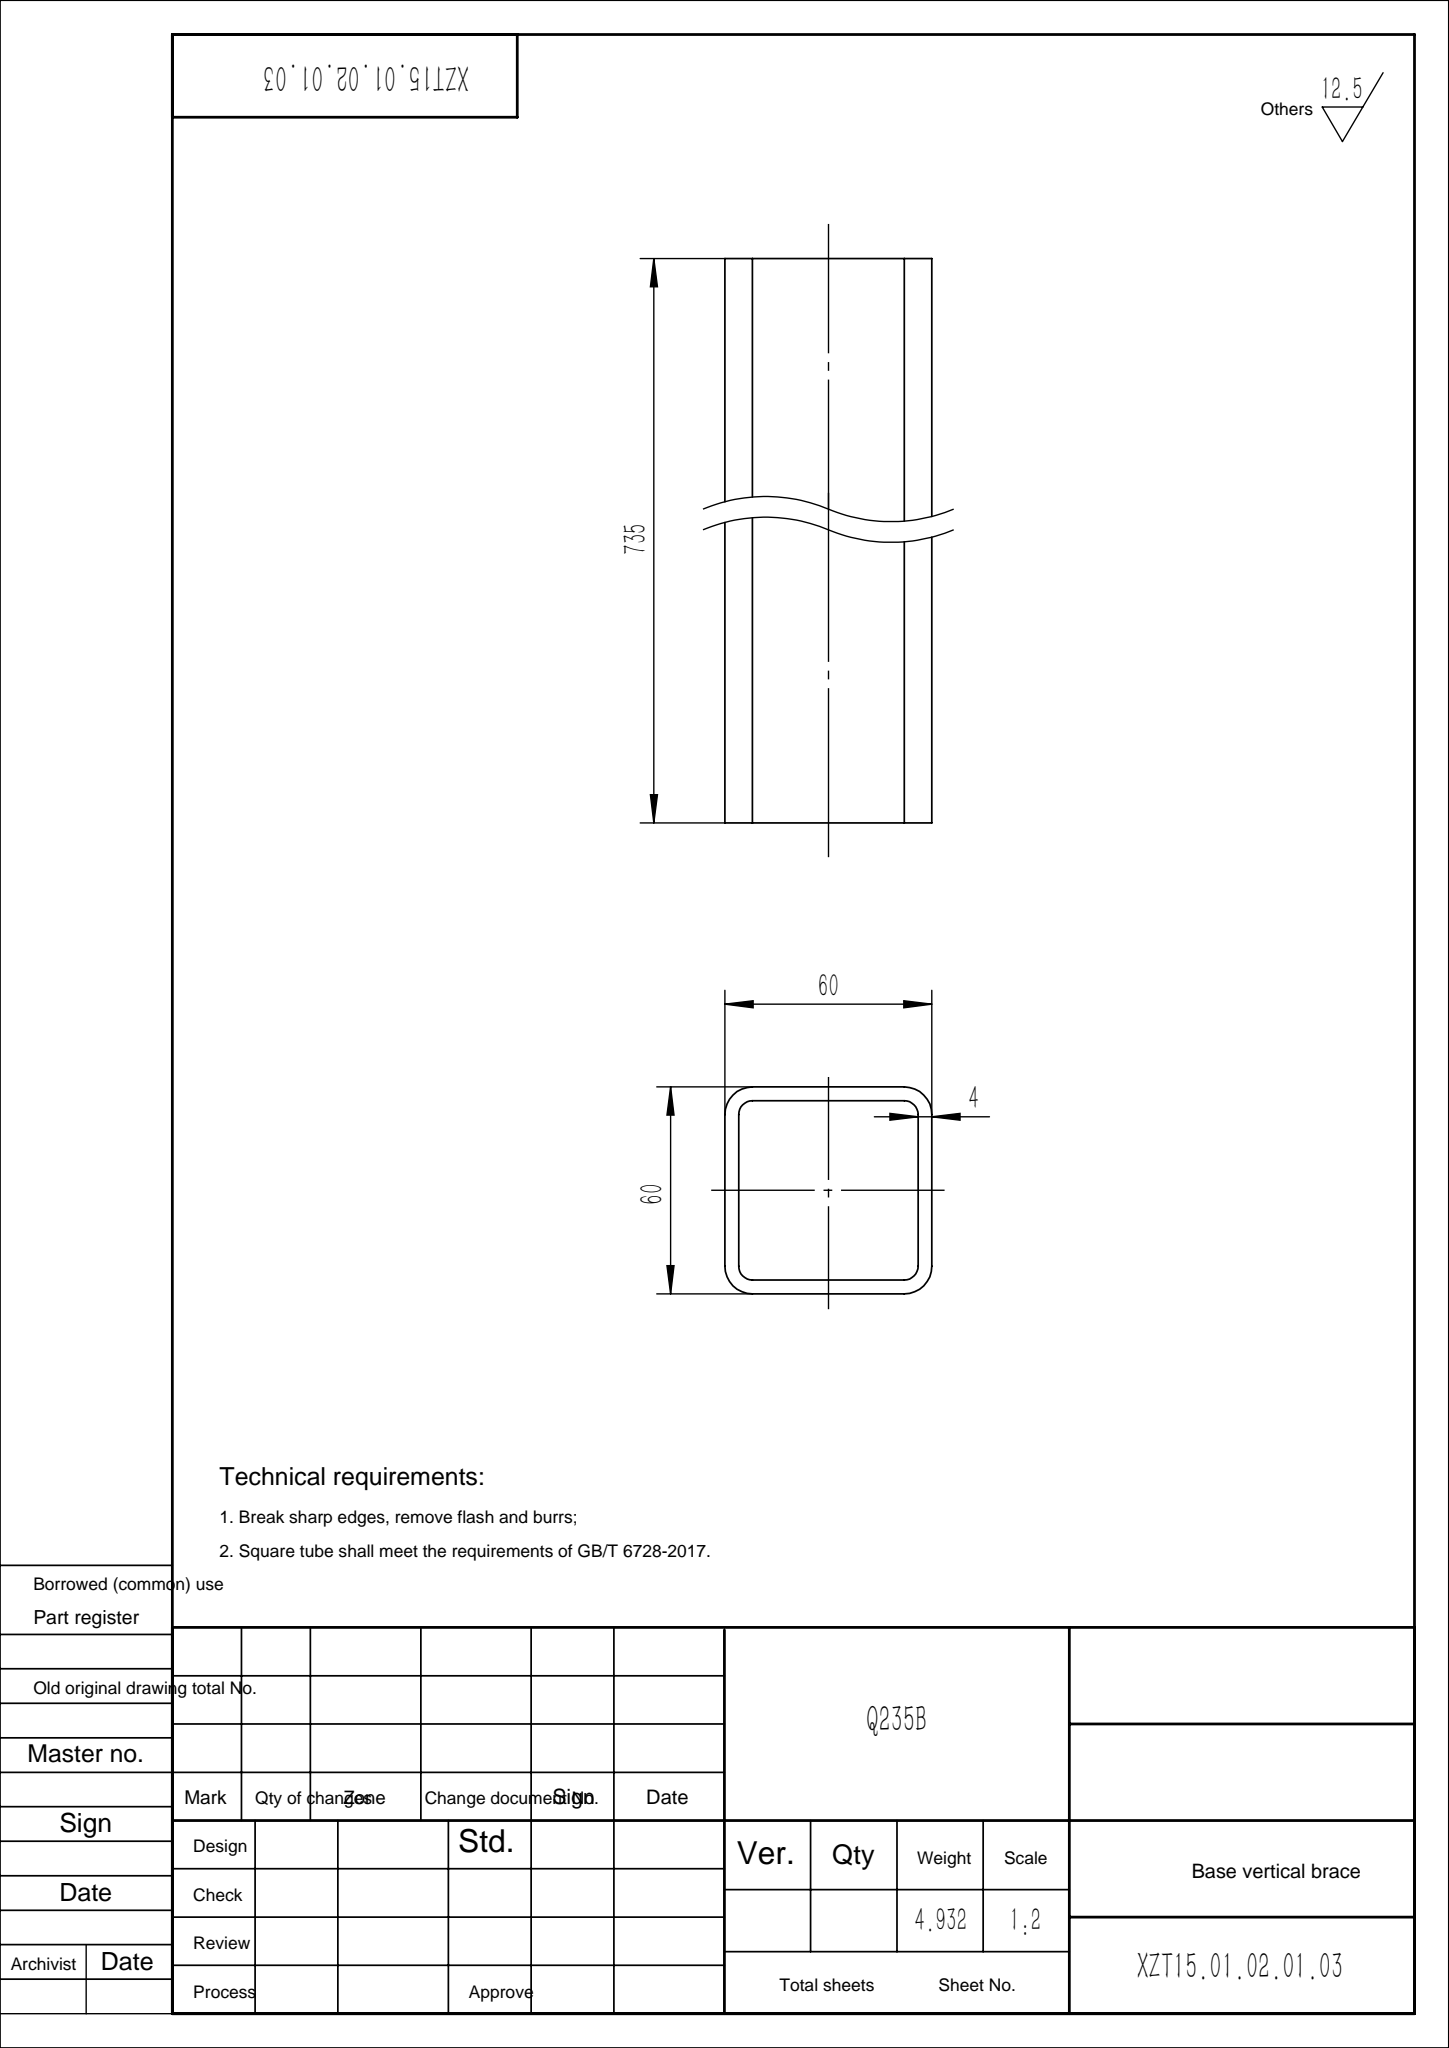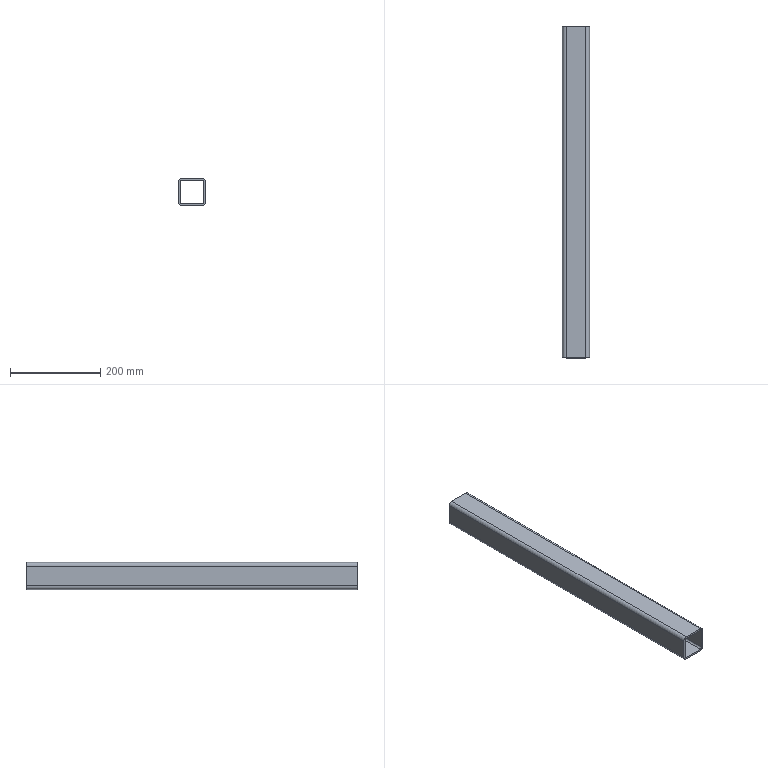Part | SolidWorks | features WeldMemberFeat 1, WeldmentFeature 1 | 1 solid | 18 faces | box 60 x 735 x 60 mm | volume 628275 mm3 | plane 10 | cylinder 8 | commonest cylinder face diameters 8 x4 16 x4
STEP:
#1=CARTESIAN_POINT('',(-30.,0.,22.));
#2=VERTEX_POINT('',#1);
#3=CARTESIAN_POINT('',(-22.,0.,30.));
#4=VERTEX_POINT('',#3);
#5=CARTESIAN_POINT('',(-22.,0.,22.));
#6=DIRECTION('',(0.,1.,0.));
#7=DIRECTION('',(0.,0.,1.));
#8=AXIS2_PLACEMENT_3D('',#5,#6,#7);
#9=CIRCLE('',#8,8.);
#10=EDGE_CURVE('',#2,#4,#9,.T.);
#11=ORIENTED_EDGE('',*,*,#10,.T.);
#12=CARTESIAN_POINT('',(-22.,735.,30.));
#13=VERTEX_POINT('',#12);
#14=CARTESIAN_POINT('',(-22.,735.,30.));
#15=DIRECTION('',(0.,-1.,0.));
#16=VECTOR('',#15,1000.);
#17=LINE('',#14,#16);
#18=EDGE_CURVE('',#13,#4,#17,.T.);
#19=ORIENTED_EDGE('',*,*,#18,.F.);
#20=CARTESIAN_POINT('',(-30.,735.,22.));
#21=VERTEX_POINT('',#20);
#22=CARTESIAN_POINT('',(-22.,735.,22.));
#23=DIRECTION('',(0.,1.,0.));
#24=DIRECTION('',(0.,0.,1.));
#25=AXIS2_PLACEMENT_3D('',#22,#23,#24);
#26=CIRCLE('',#25,8.);
#27=EDGE_CURVE('',#21,#13,#26,.T.);
#28=ORIENTED_EDGE('',*,*,#27,.F.);
#29=CARTESIAN_POINT('',(-30.,735.,22.));
#30=DIRECTION('',(0.,-1.,0.));
#31=VECTOR('',#30,1000.);
#32=LINE('',#29,#31);
#33=EDGE_CURVE('',#21,#2,#32,.T.);
#34=ORIENTED_EDGE('',*,*,#33,.T.);
#35=EDGE_LOOP('',(#11,#19,#28,#34));
#36=FACE_OUTER_BOUND('',#35,.T.);
#37=CARTESIAN_POINT('',(-22.,735.,22.));
#38=DIRECTION('',(0.,-1.,0.));
#39=DIRECTION('',(0.,0.,-1.));
#40=AXIS2_PLACEMENT_3D('',#37,#38,#39);
#41=CYLINDRICAL_SURFACE('',#40,8.);
#42=ADVANCED_FACE('',(#36),#41,.T.);
#43=CARTESIAN_POINT('',(22.,0.,30.));
#44=VERTEX_POINT('',#43);
#45=CARTESIAN_POINT('',(-22.,0.,30.));
#46=DIRECTION('',(1.,0.,0.));
#47=VECTOR('',#46,1000.);
#48=LINE('',#45,#47);
#49=EDGE_CURVE('',#4,#44,#48,.T.);
#50=ORIENTED_EDGE('',*,*,#49,.T.);
#51=CARTESIAN_POINT('',(22.,735.,30.));
#52=VERTEX_POINT('',#51);
#53=CARTESIAN_POINT('',(22.,735.,30.));
#54=DIRECTION('',(0.,-1.,0.));
#55=VECTOR('',#54,1000.);
#56=LINE('',#53,#55);
#57=EDGE_CURVE('',#52,#44,#56,.T.);
#58=ORIENTED_EDGE('',*,*,#57,.F.);
#59=CARTESIAN_POINT('',(-22.,735.,30.));
#60=DIRECTION('',(1.,0.,0.));
#61=VECTOR('',#60,1000.);
#62=LINE('',#59,#61);
#63=EDGE_CURVE('',#13,#52,#62,.T.);
#64=ORIENTED_EDGE('',*,*,#63,.F.);
#65=ORIENTED_EDGE('',*,*,#18,.T.);
#66=EDGE_LOOP('',(#50,#58,#64,#65));
#67=FACE_OUTER_BOUND('',#66,.T.);
#68=CARTESIAN_POINT('',(-22.,735.,30.));
#69=DIRECTION('',(0.,0.,-1.));
#70=DIRECTION('',(-1.,0.,0.));
#71=AXIS2_PLACEMENT_3D('',#68,#69,#70);
#72=PLANE('',#71);
#73=ADVANCED_FACE('',(#67),#72,.F.);
#74=CARTESIAN_POINT('',(30.,0.,22.));
#75=VERTEX_POINT('',#74);
#76=CARTESIAN_POINT('',(22.,0.,22.));
#77=DIRECTION('',(0.,1.,0.));
#78=DIRECTION('',(0.,0.,1.));
#79=AXIS2_PLACEMENT_3D('',#76,#77,#78);
#80=CIRCLE('',#79,8.);
#81=EDGE_CURVE('',#44,#75,#80,.T.);
#82=ORIENTED_EDGE('',*,*,#81,.T.);
#83=CARTESIAN_POINT('',(30.,735.,22.));
#84=VERTEX_POINT('',#83);
#85=CARTESIAN_POINT('',(30.,735.,22.));
#86=DIRECTION('',(0.,-1.,0.));
#87=VECTOR('',#86,1000.);
#88=LINE('',#85,#87);
#89=EDGE_CURVE('',#84,#75,#88,.T.);
#90=ORIENTED_EDGE('',*,*,#89,.F.);
#91=CARTESIAN_POINT('',(22.,735.,22.));
#92=DIRECTION('',(0.,1.,0.));
#93=DIRECTION('',(0.,0.,1.));
#94=AXIS2_PLACEMENT_3D('',#91,#92,#93);
#95=CIRCLE('',#94,8.);
#96=EDGE_CURVE('',#52,#84,#95,.T.);
#97=ORIENTED_EDGE('',*,*,#96,.F.);
#98=ORIENTED_EDGE('',*,*,#57,.T.);
#99=EDGE_LOOP('',(#82,#90,#97,#98));
#100=FACE_OUTER_BOUND('',#99,.T.);
#101=CARTESIAN_POINT('',(22.,735.,22.));
#102=DIRECTION('',(0.,-1.,0.));
#103=DIRECTION('',(0.,0.,-1.));
#104=AXIS2_PLACEMENT_3D('',#101,#102,#103);
#105=CYLINDRICAL_SURFACE('',#104,8.);
#106=ADVANCED_FACE('',(#100),#105,.T.);
#107=CARTESIAN_POINT('',(30.,0.,-22.));
#108=VERTEX_POINT('',#107);
#109=CARTESIAN_POINT('',(30.,0.,-22.));
#110=DIRECTION('',(0.,0.,-1.));
#111=VECTOR('',#110,1000.);
#112=LINE('',#109,#111);
#113=EDGE_CURVE('',#75,#108,#112,.T.);
#114=ORIENTED_EDGE('',*,*,#113,.T.);
#115=CARTESIAN_POINT('',(30.,735.,-22.));
#116=VERTEX_POINT('',#115);
#117=CARTESIAN_POINT('',(30.,735.,-22.));
#118=DIRECTION('',(0.,-1.,0.));
#119=VECTOR('',#118,1000.);
#120=LINE('',#117,#119);
#121=EDGE_CURVE('',#116,#108,#120,.T.);
#122=ORIENTED_EDGE('',*,*,#121,.F.);
#123=CARTESIAN_POINT('',(30.,735.,-22.));
#124=DIRECTION('',(0.,0.,-1.));
#125=VECTOR('',#124,1000.);
#126=LINE('',#123,#125);
#127=EDGE_CURVE('',#84,#116,#126,.T.);
#128=ORIENTED_EDGE('',*,*,#127,.F.);
#129=ORIENTED_EDGE('',*,*,#89,.T.);
#130=EDGE_LOOP('',(#114,#122,#128,#129));
#131=FACE_OUTER_BOUND('',#130,.T.);
#132=CARTESIAN_POINT('',(30.,735.,-22.));
#133=DIRECTION('',(-1.,0.,0.));
#134=DIRECTION('',(0.,0.,1.));
#135=AXIS2_PLACEMENT_3D('',#132,#133,#134);
#136=PLANE('',#135);
#137=ADVANCED_FACE('',(#131),#136,.F.);
#138=CARTESIAN_POINT('',(22.,0.,-30.));
#139=VERTEX_POINT('',#138);
#140=CARTESIAN_POINT('',(22.,0.,-22.));
#141=DIRECTION('',(0.,1.,0.));
#142=DIRECTION('',(0.,0.,1.));
#143=AXIS2_PLACEMENT_3D('',#140,#141,#142);
#144=CIRCLE('',#143,8.);
#145=EDGE_CURVE('',#108,#139,#144,.T.);
#146=ORIENTED_EDGE('',*,*,#145,.T.);
#147=CARTESIAN_POINT('',(22.,735.,-30.));
#148=VERTEX_POINT('',#147);
#149=CARTESIAN_POINT('',(22.,735.,-30.));
#150=DIRECTION('',(0.,-1.,0.));
#151=VECTOR('',#150,1000.);
#152=LINE('',#149,#151);
#153=EDGE_CURVE('',#148,#139,#152,.T.);
#154=ORIENTED_EDGE('',*,*,#153,.F.);
#155=CARTESIAN_POINT('',(22.,735.,-22.));
#156=DIRECTION('',(0.,1.,0.));
#157=DIRECTION('',(0.,0.,1.));
#158=AXIS2_PLACEMENT_3D('',#155,#156,#157);
#159=CIRCLE('',#158,8.);
#160=EDGE_CURVE('',#116,#148,#159,.T.);
#161=ORIENTED_EDGE('',*,*,#160,.F.);
#162=ORIENTED_EDGE('',*,*,#121,.T.);
#163=EDGE_LOOP('',(#146,#154,#161,#162));
#164=FACE_OUTER_BOUND('',#163,.T.);
#165=CARTESIAN_POINT('',(22.,735.,-22.));
#166=DIRECTION('',(0.,-1.,0.));
#167=DIRECTION('',(0.,0.,-1.));
#168=AXIS2_PLACEMENT_3D('',#165,#166,#167);
#169=CYLINDRICAL_SURFACE('',#168,8.);
#170=ADVANCED_FACE('',(#164),#169,.T.);
#171=CARTESIAN_POINT('',(-22.,0.,-30.));
#172=VERTEX_POINT('',#171);
#173=CARTESIAN_POINT('',(22.,0.,-30.));
#174=DIRECTION('',(-1.,0.,0.));
#175=VECTOR('',#174,1000.);
#176=LINE('',#173,#175);
#177=EDGE_CURVE('',#139,#172,#176,.T.);
#178=ORIENTED_EDGE('',*,*,#177,.T.);
#179=CARTESIAN_POINT('',(-22.,735.,-30.));
#180=VERTEX_POINT('',#179);
#181=CARTESIAN_POINT('',(-22.,735.,-30.));
#182=DIRECTION('',(0.,-1.,0.));
#183=VECTOR('',#182,1000.);
#184=LINE('',#181,#183);
#185=EDGE_CURVE('',#180,#172,#184,.T.);
#186=ORIENTED_EDGE('',*,*,#185,.F.);
#187=CARTESIAN_POINT('',(22.,735.,-30.));
#188=DIRECTION('',(-1.,0.,0.));
#189=VECTOR('',#188,1000.);
#190=LINE('',#187,#189);
#191=EDGE_CURVE('',#148,#180,#190,.T.);
#192=ORIENTED_EDGE('',*,*,#191,.F.);
#193=ORIENTED_EDGE('',*,*,#153,.T.);
#194=EDGE_LOOP('',(#178,#186,#192,#193));
#195=FACE_OUTER_BOUND('',#194,.T.);
#196=CARTESIAN_POINT('',(22.,735.,-30.));
#197=DIRECTION('',(0.,0.,1.));
#198=DIRECTION('',(1.,0.,0.));
#199=AXIS2_PLACEMENT_3D('',#196,#197,#198);
#200=PLANE('',#199);
#201=ADVANCED_FACE('',(#195),#200,.F.);
#202=CARTESIAN_POINT('',(-30.,0.,-22.));
#203=VERTEX_POINT('',#202);
#204=CARTESIAN_POINT('',(-22.,0.,-22.));
#205=DIRECTION('',(0.,1.,0.));
#206=DIRECTION('',(0.,0.,1.));
#207=AXIS2_PLACEMENT_3D('',#204,#205,#206);
#208=CIRCLE('',#207,8.);
#209=EDGE_CURVE('',#172,#203,#208,.T.);
#210=ORIENTED_EDGE('',*,*,#209,.T.);
#211=CARTESIAN_POINT('',(-30.,735.,-22.));
#212=VERTEX_POINT('',#211);
#213=CARTESIAN_POINT('',(-30.,735.,-22.));
#214=DIRECTION('',(0.,-1.,0.));
#215=VECTOR('',#214,1000.);
#216=LINE('',#213,#215);
#217=EDGE_CURVE('',#212,#203,#216,.T.);
#218=ORIENTED_EDGE('',*,*,#217,.F.);
#219=CARTESIAN_POINT('',(-22.,735.,-22.));
#220=DIRECTION('',(0.,1.,0.));
#221=DIRECTION('',(0.,0.,1.));
#222=AXIS2_PLACEMENT_3D('',#219,#220,#221);
#223=CIRCLE('',#222,8.);
#224=EDGE_CURVE('',#180,#212,#223,.T.);
#225=ORIENTED_EDGE('',*,*,#224,.F.);
#226=ORIENTED_EDGE('',*,*,#185,.T.);
#227=EDGE_LOOP('',(#210,#218,#225,#226));
#228=FACE_OUTER_BOUND('',#227,.T.);
#229=CARTESIAN_POINT('',(-22.,735.,-22.));
#230=DIRECTION('',(0.,-1.,0.));
#231=DIRECTION('',(0.,0.,-1.));
#232=AXIS2_PLACEMENT_3D('',#229,#230,#231);
#233=CYLINDRICAL_SURFACE('',#232,8.);
#234=ADVANCED_FACE('',(#228),#233,.T.);
#235=CARTESIAN_POINT('',(22.,0.,26.));
#236=VERTEX_POINT('',#235);
#237=CARTESIAN_POINT('',(26.,0.,22.));
#238=VERTEX_POINT('',#237);
#239=CARTESIAN_POINT('',(22.,0.,22.));
#240=DIRECTION('',(0.,1.,0.));
#241=DIRECTION('',(0.,0.,1.));
#242=AXIS2_PLACEMENT_3D('',#239,#240,#241);
#243=CIRCLE('',#242,4.);
#244=EDGE_CURVE('',#236,#238,#243,.T.);
#245=ORIENTED_EDGE('',*,*,#244,.F.);
#246=CARTESIAN_POINT('',(22.,735.,26.));
#247=VERTEX_POINT('',#246);
#248=CARTESIAN_POINT('',(22.,735.,26.));
#249=DIRECTION('',(0.,-1.,0.));
#250=VECTOR('',#249,1000.);
#251=LINE('',#248,#250);
#252=EDGE_CURVE('',#247,#236,#251,.T.);
#253=ORIENTED_EDGE('',*,*,#252,.F.);
#254=CARTESIAN_POINT('',(26.,735.,22.));
#255=VERTEX_POINT('',#254);
#256=CARTESIAN_POINT('',(22.,735.,22.));
#257=DIRECTION('',(0.,1.,0.));
#258=DIRECTION('',(0.,0.,1.));
#259=AXIS2_PLACEMENT_3D('',#256,#257,#258);
#260=CIRCLE('',#259,4.);
#261=EDGE_CURVE('',#247,#255,#260,.T.);
#262=ORIENTED_EDGE('',*,*,#261,.T.);
#263=CARTESIAN_POINT('',(26.,735.,22.));
#264=DIRECTION('',(0.,-1.,0.));
#265=VECTOR('',#264,1000.);
#266=LINE('',#263,#265);
#267=EDGE_CURVE('',#255,#238,#266,.T.);
#268=ORIENTED_EDGE('',*,*,#267,.T.);
#269=EDGE_LOOP('',(#245,#253,#262,#268));
#270=FACE_OUTER_BOUND('',#269,.T.);
#271=CARTESIAN_POINT('',(22.,735.,22.));
#272=DIRECTION('',(0.,-1.,0.));
#273=DIRECTION('',(0.,0.,-1.));
#274=AXIS2_PLACEMENT_3D('',#271,#272,#273);
#275=CYLINDRICAL_SURFACE('',#274,4.);
#276=ADVANCED_FACE('',(#270),#275,.F.);
#277=CARTESIAN_POINT('',(-22.,0.,26.));
#278=VERTEX_POINT('',#277);
#279=CARTESIAN_POINT('',(-22.,0.,26.));
#280=DIRECTION('',(1.,0.,0.));
#281=VECTOR('',#280,1000.);
#282=LINE('',#279,#281);
#283=EDGE_CURVE('',#278,#236,#282,.T.);
#284=ORIENTED_EDGE('',*,*,#283,.F.);
#285=CARTESIAN_POINT('',(-22.,735.,26.));
#286=VERTEX_POINT('',#285);
#287=CARTESIAN_POINT('',(-22.,735.,26.));
#288=DIRECTION('',(0.,-1.,0.));
#289=VECTOR('',#288,1000.);
#290=LINE('',#287,#289);
#291=EDGE_CURVE('',#286,#278,#290,.T.);
#292=ORIENTED_EDGE('',*,*,#291,.F.);
#293=CARTESIAN_POINT('',(-22.,735.,26.));
#294=DIRECTION('',(1.,0.,0.));
#295=VECTOR('',#294,1000.);
#296=LINE('',#293,#295);
#297=EDGE_CURVE('',#286,#247,#296,.T.);
#298=ORIENTED_EDGE('',*,*,#297,.T.);
#299=ORIENTED_EDGE('',*,*,#252,.T.);
#300=EDGE_LOOP('',(#284,#292,#298,#299));
#301=FACE_OUTER_BOUND('',#300,.T.);
#302=CARTESIAN_POINT('',(-22.,735.,26.));
#303=DIRECTION('',(0.,0.,-1.));
#304=DIRECTION('',(-1.,0.,0.));
#305=AXIS2_PLACEMENT_3D('',#302,#303,#304);
#306=PLANE('',#305);
#307=ADVANCED_FACE('',(#301),#306,.T.);
#308=CARTESIAN_POINT('',(-26.,0.,22.));
#309=VERTEX_POINT('',#308);
#310=CARTESIAN_POINT('',(-22.,0.,22.));
#311=DIRECTION('',(0.,1.,0.));
#312=DIRECTION('',(0.,0.,1.));
#313=AXIS2_PLACEMENT_3D('',#310,#311,#312);
#314=CIRCLE('',#313,4.);
#315=EDGE_CURVE('',#309,#278,#314,.T.);
#316=ORIENTED_EDGE('',*,*,#315,.F.);
#317=CARTESIAN_POINT('',(-26.,735.,22.));
#318=VERTEX_POINT('',#317);
#319=CARTESIAN_POINT('',(-26.,735.,22.));
#320=DIRECTION('',(0.,-1.,0.));
#321=VECTOR('',#320,1000.);
#322=LINE('',#319,#321);
#323=EDGE_CURVE('',#318,#309,#322,.T.);
#324=ORIENTED_EDGE('',*,*,#323,.F.);
#325=CARTESIAN_POINT('',(-22.,735.,22.));
#326=DIRECTION('',(0.,1.,0.));
#327=DIRECTION('',(0.,0.,1.));
#328=AXIS2_PLACEMENT_3D('',#325,#326,#327);
#329=CIRCLE('',#328,4.);
#330=EDGE_CURVE('',#318,#286,#329,.T.);
#331=ORIENTED_EDGE('',*,*,#330,.T.);
#332=ORIENTED_EDGE('',*,*,#291,.T.);
#333=EDGE_LOOP('',(#316,#324,#331,#332));
#334=FACE_OUTER_BOUND('',#333,.T.);
#335=CARTESIAN_POINT('',(-22.,735.,22.));
#336=DIRECTION('',(0.,-1.,0.));
#337=DIRECTION('',(0.,0.,-1.));
#338=AXIS2_PLACEMENT_3D('',#335,#336,#337);
#339=CYLINDRICAL_SURFACE('',#338,4.);
#340=ADVANCED_FACE('',(#334),#339,.F.);
#341=CARTESIAN_POINT('',(-26.,0.,-22.));
#342=VERTEX_POINT('',#341);
#343=CARTESIAN_POINT('',(-26.,0.,22.));
#344=DIRECTION('',(0.,0.,1.));
#345=VECTOR('',#344,1000.);
#346=LINE('',#343,#345);
#347=EDGE_CURVE('',#342,#309,#346,.T.);
#348=ORIENTED_EDGE('',*,*,#347,.F.);
#349=CARTESIAN_POINT('',(-26.,735.,-22.));
#350=VERTEX_POINT('',#349);
#351=CARTESIAN_POINT('',(-26.,735.,-22.));
#352=DIRECTION('',(0.,-1.,0.));
#353=VECTOR('',#352,1000.);
#354=LINE('',#351,#353);
#355=EDGE_CURVE('',#350,#342,#354,.T.);
#356=ORIENTED_EDGE('',*,*,#355,.F.);
#357=CARTESIAN_POINT('',(-26.,735.,22.));
#358=DIRECTION('',(0.,0.,1.));
#359=VECTOR('',#358,1000.);
#360=LINE('',#357,#359);
#361=EDGE_CURVE('',#350,#318,#360,.T.);
#362=ORIENTED_EDGE('',*,*,#361,.T.);
#363=ORIENTED_EDGE('',*,*,#323,.T.);
#364=EDGE_LOOP('',(#348,#356,#362,#363));
#365=FACE_OUTER_BOUND('',#364,.T.);
#366=CARTESIAN_POINT('',(-26.,735.,22.));
#367=DIRECTION('',(1.,0.,0.));
#368=DIRECTION('',(0.,0.,-1.));
#369=AXIS2_PLACEMENT_3D('',#366,#367,#368);
#370=PLANE('',#369);
#371=ADVANCED_FACE('',(#365),#370,.T.);
#372=CARTESIAN_POINT('',(-22.,0.,-26.));
#373=VERTEX_POINT('',#372);
#374=CARTESIAN_POINT('',(-22.,0.,-22.));
#375=DIRECTION('',(0.,1.,0.));
#376=DIRECTION('',(0.,0.,1.));
#377=AXIS2_PLACEMENT_3D('',#374,#375,#376);
#378=CIRCLE('',#377,4.);
#379=EDGE_CURVE('',#373,#342,#378,.T.);
#380=ORIENTED_EDGE('',*,*,#379,.F.);
#381=CARTESIAN_POINT('',(-22.,735.,-26.));
#382=VERTEX_POINT('',#381);
#383=CARTESIAN_POINT('',(-22.,735.,-26.));
#384=DIRECTION('',(0.,-1.,0.));
#385=VECTOR('',#384,1000.);
#386=LINE('',#383,#385);
#387=EDGE_CURVE('',#382,#373,#386,.T.);
#388=ORIENTED_EDGE('',*,*,#387,.F.);
#389=CARTESIAN_POINT('',(-22.,735.,-22.));
#390=DIRECTION('',(0.,1.,0.));
#391=DIRECTION('',(0.,0.,1.));
#392=AXIS2_PLACEMENT_3D('',#389,#390,#391);
#393=CIRCLE('',#392,4.);
#394=EDGE_CURVE('',#382,#350,#393,.T.);
#395=ORIENTED_EDGE('',*,*,#394,.T.);
#396=ORIENTED_EDGE('',*,*,#355,.T.);
#397=EDGE_LOOP('',(#380,#388,#395,#396));
#398=FACE_OUTER_BOUND('',#397,.T.);
#399=CARTESIAN_POINT('',(-22.,735.,-22.));
#400=DIRECTION('',(0.,-1.,0.));
#401=DIRECTION('',(0.,0.,-1.));
#402=AXIS2_PLACEMENT_3D('',#399,#400,#401);
#403=CYLINDRICAL_SURFACE('',#402,4.);
#404=ADVANCED_FACE('',(#398),#403,.F.);
#405=CARTESIAN_POINT('',(22.,0.,-26.));
#406=VERTEX_POINT('',#405);
#407=CARTESIAN_POINT('',(22.,0.,-26.));
#408=DIRECTION('',(-1.,0.,0.));
#409=VECTOR('',#408,1000.);
#410=LINE('',#407,#409);
#411=EDGE_CURVE('',#406,#373,#410,.T.);
#412=ORIENTED_EDGE('',*,*,#411,.F.);
#413=CARTESIAN_POINT('',(22.,735.,-26.));
#414=VERTEX_POINT('',#413);
#415=CARTESIAN_POINT('',(22.,735.,-26.));
#416=DIRECTION('',(0.,-1.,0.));
#417=VECTOR('',#416,1000.);
#418=LINE('',#415,#417);
#419=EDGE_CURVE('',#414,#406,#418,.T.);
#420=ORIENTED_EDGE('',*,*,#419,.F.);
#421=CARTESIAN_POINT('',(22.,735.,-26.));
#422=DIRECTION('',(-1.,0.,0.));
#423=VECTOR('',#422,1000.);
#424=LINE('',#421,#423);
#425=EDGE_CURVE('',#414,#382,#424,.T.);
#426=ORIENTED_EDGE('',*,*,#425,.T.);
#427=ORIENTED_EDGE('',*,*,#387,.T.);
#428=EDGE_LOOP('',(#412,#420,#426,#427));
#429=FACE_OUTER_BOUND('',#428,.T.);
#430=CARTESIAN_POINT('',(22.,735.,-26.));
#431=DIRECTION('',(0.,0.,1.));
#432=DIRECTION('',(1.,0.,0.));
#433=AXIS2_PLACEMENT_3D('',#430,#431,#432);
#434=PLANE('',#433);
#435=ADVANCED_FACE('',(#429),#434,.T.);
#436=CARTESIAN_POINT('',(26.,0.,-22.));
#437=VERTEX_POINT('',#436);
#438=CARTESIAN_POINT('',(22.,0.,-22.));
#439=DIRECTION('',(0.,1.,0.));
#440=DIRECTION('',(0.,0.,1.));
#441=AXIS2_PLACEMENT_3D('',#438,#439,#440);
#442=CIRCLE('',#441,4.);
#443=EDGE_CURVE('',#437,#406,#442,.T.);
#444=ORIENTED_EDGE('',*,*,#443,.F.);
#445=CARTESIAN_POINT('',(26.,735.,-22.));
#446=VERTEX_POINT('',#445);
#447=CARTESIAN_POINT('',(26.,735.,-22.));
#448=DIRECTION('',(0.,-1.,0.));
#449=VECTOR('',#448,1000.);
#450=LINE('',#447,#449);
#451=EDGE_CURVE('',#446,#437,#450,.T.);
#452=ORIENTED_EDGE('',*,*,#451,.F.);
#453=CARTESIAN_POINT('',(22.,735.,-22.));
#454=DIRECTION('',(0.,1.,0.));
#455=DIRECTION('',(0.,0.,1.));
#456=AXIS2_PLACEMENT_3D('',#453,#454,#455);
#457=CIRCLE('',#456,4.);
#458=EDGE_CURVE('',#446,#414,#457,.T.);
#459=ORIENTED_EDGE('',*,*,#458,.T.);
#460=ORIENTED_EDGE('',*,*,#419,.T.);
#461=EDGE_LOOP('',(#444,#452,#459,#460));
#462=FACE_OUTER_BOUND('',#461,.T.);
#463=CARTESIAN_POINT('',(22.,735.,-22.));
#464=DIRECTION('',(0.,-1.,0.));
#465=DIRECTION('',(0.,0.,-1.));
#466=AXIS2_PLACEMENT_3D('',#463,#464,#465);
#467=CYLINDRICAL_SURFACE('',#466,4.);
#468=ADVANCED_FACE('',(#462),#467,.F.);
#469=CARTESIAN_POINT('',(26.,0.,-22.));
#470=DIRECTION('',(0.,0.,-1.));
#471=VECTOR('',#470,1000.);
#472=LINE('',#469,#471);
#473=EDGE_CURVE('',#238,#437,#472,.T.);
#474=ORIENTED_EDGE('',*,*,#473,.F.);
#475=ORIENTED_EDGE('',*,*,#267,.F.);
#476=CARTESIAN_POINT('',(26.,735.,-22.));
#477=DIRECTION('',(0.,0.,-1.));
#478=VECTOR('',#477,1000.);
#479=LINE('',#476,#478);
#480=EDGE_CURVE('',#255,#446,#479,.T.);
#481=ORIENTED_EDGE('',*,*,#480,.T.);
#482=ORIENTED_EDGE('',*,*,#451,.T.);
#483=EDGE_LOOP('',(#474,#475,#481,#482));
#484=FACE_OUTER_BOUND('',#483,.T.);
#485=CARTESIAN_POINT('',(26.,735.,-22.));
#486=DIRECTION('',(-1.,0.,0.));
#487=DIRECTION('',(0.,0.,1.));
#488=AXIS2_PLACEMENT_3D('',#485,#486,#487);
#489=PLANE('',#488);
#490=ADVANCED_FACE('',(#484),#489,.T.);
#491=CARTESIAN_POINT('',(-30.,0.,22.));
#492=DIRECTION('',(0.,0.,1.));
#493=VECTOR('',#492,1000.);
#494=LINE('',#491,#493);
#495=EDGE_CURVE('',#203,#2,#494,.T.);
#496=ORIENTED_EDGE('',*,*,#495,.T.);
#497=ORIENTED_EDGE('',*,*,#33,.F.);
#498=CARTESIAN_POINT('',(-30.,735.,22.));
#499=DIRECTION('',(0.,0.,1.));
#500=VECTOR('',#499,1000.);
#501=LINE('',#498,#500);
#502=EDGE_CURVE('',#212,#21,#501,.T.);
#503=ORIENTED_EDGE('',*,*,#502,.F.);
#504=ORIENTED_EDGE('',*,*,#217,.T.);
#505=EDGE_LOOP('',(#496,#497,#503,#504));
#506=FACE_OUTER_BOUND('',#505,.T.);
#507=CARTESIAN_POINT('',(-30.,735.,22.));
#508=DIRECTION('',(1.,0.,0.));
#509=DIRECTION('',(0.,0.,-1.));
#510=AXIS2_PLACEMENT_3D('',#507,#508,#509);
#511=PLANE('',#510);
#512=ADVANCED_FACE('',(#506),#511,.F.);
#513=ORIENTED_EDGE('',*,*,#261,.F.);
#514=ORIENTED_EDGE('',*,*,#297,.F.);
#515=ORIENTED_EDGE('',*,*,#330,.F.);
#516=ORIENTED_EDGE('',*,*,#361,.F.);
#517=ORIENTED_EDGE('',*,*,#394,.F.);
#518=ORIENTED_EDGE('',*,*,#425,.F.);
#519=ORIENTED_EDGE('',*,*,#458,.F.);
#520=ORIENTED_EDGE('',*,*,#480,.F.);
#521=EDGE_LOOP('',(#513,#514,#515,#516,#517,#518,#519,#520));
#522=FACE_BOUND('',#521,.T.);
#523=ORIENTED_EDGE('',*,*,#27,.T.);
#524=ORIENTED_EDGE('',*,*,#63,.T.);
#525=ORIENTED_EDGE('',*,*,#96,.T.);
#526=ORIENTED_EDGE('',*,*,#127,.T.);
#527=ORIENTED_EDGE('',*,*,#160,.T.);
#528=ORIENTED_EDGE('',*,*,#191,.T.);
#529=ORIENTED_EDGE('',*,*,#224,.T.);
#530=ORIENTED_EDGE('',*,*,#502,.T.);
#531=EDGE_LOOP('',(#523,#524,#525,#526,#527,#528,#529,#530));
#532=FACE_OUTER_BOUND('',#531,.T.);
#533=CARTESIAN_POINT('',(-22.,735.,22.));
#534=DIRECTION('',(0.,1.,0.));
#535=DIRECTION('',(0.,0.,1.));
#536=AXIS2_PLACEMENT_3D('',#533,#534,#535);
#537=PLANE('',#536);
#538=ADVANCED_FACE('',(#522,#532),#537,.T.);
#539=ORIENTED_EDGE('',*,*,#244,.T.);
#540=ORIENTED_EDGE('',*,*,#473,.T.);
#541=ORIENTED_EDGE('',*,*,#443,.T.);
#542=ORIENTED_EDGE('',*,*,#411,.T.);
#543=ORIENTED_EDGE('',*,*,#379,.T.);
#544=ORIENTED_EDGE('',*,*,#347,.T.);
#545=ORIENTED_EDGE('',*,*,#315,.T.);
#546=ORIENTED_EDGE('',*,*,#283,.T.);
#547=EDGE_LOOP('',(#539,#540,#541,#542,#543,#544,#545,#546));
#548=FACE_BOUND('',#547,.T.);
#549=ORIENTED_EDGE('',*,*,#10,.F.);
#550=ORIENTED_EDGE('',*,*,#495,.F.);
#551=ORIENTED_EDGE('',*,*,#209,.F.);
#552=ORIENTED_EDGE('',*,*,#177,.F.);
#553=ORIENTED_EDGE('',*,*,#145,.F.);
#554=ORIENTED_EDGE('',*,*,#113,.F.);
#555=ORIENTED_EDGE('',*,*,#81,.F.);
#556=ORIENTED_EDGE('',*,*,#49,.F.);
#557=EDGE_LOOP('',(#549,#550,#551,#552,#553,#554,#555,#556));
#558=FACE_OUTER_BOUND('',#557,.T.);
#559=CARTESIAN_POINT('',(-22.,0.,22.));
#560=DIRECTION('',(0.,1.,0.));
#561=DIRECTION('',(0.,0.,1.));
#562=AXIS2_PLACEMENT_3D('',#559,#560,#561);
#563=PLANE('',#562);
#564=ADVANCED_FACE('',(#548,#558),#563,.F.);
#565=CLOSED_SHELL('',(#42,#73,#106,#137,#170,#201,#234,#276,#307,#340,#371,#404,#435,#468,#490,#512,#538,#564));
#566=MANIFOLD_SOLID_BREP('',#565);
#567=CARTESIAN_POINT('',(0.,0.,0.));
#568=DIRECTION('',(0.,0.,1.));
#569=DIRECTION('',(1.,0.,0.));
#570=AXIS2_PLACEMENT_3D('',#567,#568,#569);
#571=(LENGTH_UNIT()NAMED_UNIT(*)SI_UNIT(.MILLI.,.METRE.));
#572=UNCERTAINTY_MEASURE_WITH_UNIT(LENGTH_MEASURE(0.00001),#571,'','');
#573=(NAMED_UNIT(*)PLANE_ANGLE_UNIT()SI_UNIT($,.RADIAN.));
#574=(NAMED_UNIT(*)SI_UNIT($,.STERADIAN.)SOLID_ANGLE_UNIT());
#575=(GEOMETRIC_REPRESENTATION_CONTEXT(3)GLOBAL_UNCERTAINTY_ASSIGNED_CONTEXT((#572))GLOBAL_UNIT_ASSIGNED_CONTEXT((#571,#573,#574))REPRESENTATION_CONTEXT('',''));
#576=ADVANCED_BREP_SHAPE_REPRESENTATION('',(#566,#570),#575);